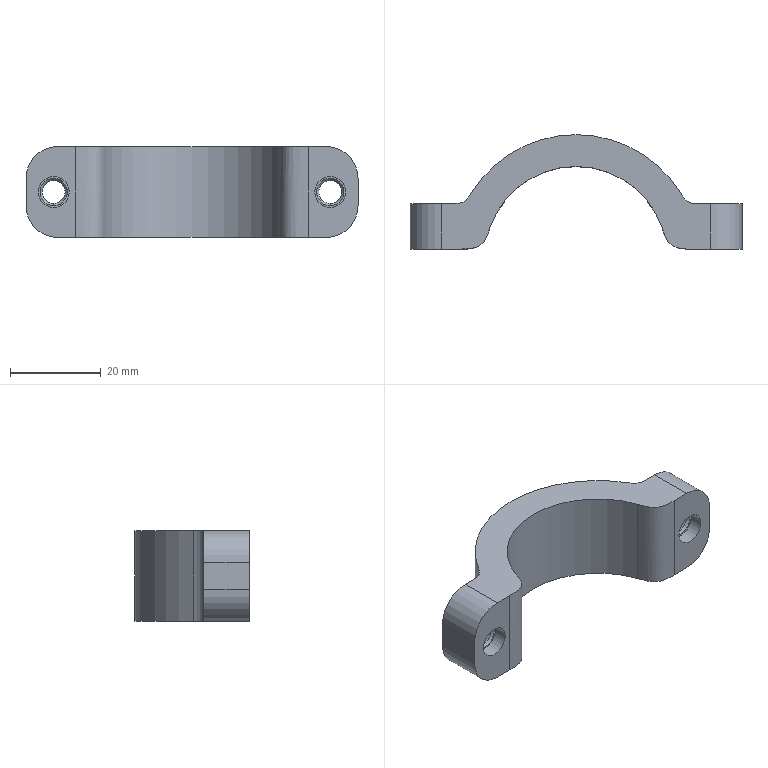Part | 1 solid | 36 faces | box 73 x 25.677 x 20 mm | volume 13024 mm3 | cylinder 14 | plane 10 | cone 8 | other 4 | commonest cylinder face diameters 5 x4 6.8 x4 14 x4 40.1 x1 54.1 x1
STEP:
#1=CARTESIAN_POINT('',(0.,0.,0.));
#2=DIRECTION('',(0.,0.,1.));
#3=DIRECTION('',(1.,0.,0.));
#4=AXIS2_PLACEMENT_3D('',#1,#2,#3);
#5=CARTESIAN_POINT('',(-22.998,-0.2208,0.000000113));
#6=VERTEX_POINT('',#5);
#7=CARTESIAN_POINT('',(-27.249,-2.588,0.000000113));
#8=VERTEX_POINT('',#7);
#9=CARTESIAN_POINT('',(-22.998,-0.2208,0.000000113));
#10=CARTESIAN_POINT('',(-23.584,-1.168,0.000000113));
#11=CARTESIAN_POINT('',(-24.122,-2.145,0.000000113));
#12=CARTESIAN_POINT('',(-25.021,-2.588,0.000000113));
#13=CARTESIAN_POINT('',(-26.135,-2.588,0.000000113));
#14=CARTESIAN_POINT('',(-27.249,-2.588,0.000000113));
#15=B_SPLINE_CURVE_WITH_KNOTS('',5,(#9,#10,#11,#12,#13,#14),.UNSPECIFIED.,.F.,.U.,(6,6),(0.,1.),.UNSPECIFIED.);
#16=EDGE_CURVE('',#6,#8,#15,.T.);
#17=ORIENTED_EDGE('',*,*,#16,.F.);
#18=CARTESIAN_POINT('',(-22.998,-0.2208,-20.));
#19=VERTEX_POINT('',#18);
#20=CARTESIAN_POINT('',(-22.998,-0.2208,-19.5));
#21=DIRECTION('',(0.,0.,1.));
#22=VECTOR('',#21,1.);
#23=LINE('',#20,#22);
#24=EDGE_CURVE('',#19,#6,#23,.T.);
#25=ORIENTED_EDGE('',*,*,#24,.F.);
#26=CARTESIAN_POINT('',(-27.249,-2.588,-20.));
#27=VERTEX_POINT('',#26);
#28=CARTESIAN_POINT('',(-22.998,-0.2208,-20.));
#29=CARTESIAN_POINT('',(-23.584,-1.168,-20.));
#30=CARTESIAN_POINT('',(-24.122,-2.145,-20.));
#31=CARTESIAN_POINT('',(-25.021,-2.588,-20.));
#32=CARTESIAN_POINT('',(-26.135,-2.588,-20.));
#33=CARTESIAN_POINT('',(-27.249,-2.588,-20.));
#34=B_SPLINE_CURVE_WITH_KNOTS('',5,(#28,#29,#30,#31,#32,#33),.UNSPECIFIED.,.F.,.U.,(6,6),(0.,1.),.UNSPECIFIED.);
#35=EDGE_CURVE('',#19,#27,#34,.T.);
#36=ORIENTED_EDGE('',*,*,#35,.T.);
#37=CARTESIAN_POINT('',(-27.249,-2.588,-19.5));
#38=DIRECTION('',(0.,0.,1.));
#39=VECTOR('',#38,1.);
#40=LINE('',#37,#39);
#41=EDGE_CURVE('',#27,#8,#40,.T.);
#42=ORIENTED_EDGE('',*,*,#41,.T.);
#43=EDGE_LOOP('',(#17,#25,#36,#42));
#44=FACE_OUTER_BOUND('',#43,.T.);
#45=CARTESIAN_POINT('',(-22.7,0.2499,-10.));
#46=CARTESIAN_POINT('',(-22.761,0.1563,-10.));
#47=CARTESIAN_POINT('',(-22.821,0.06246,-10.));
#48=CARTESIAN_POINT('',(-22.88,-0.03167,-10.));
#49=CARTESIAN_POINT('',(-23.531,-1.07,-10.));
#50=CARTESIAN_POINT('',(-24.122,-2.145,-10.));
#51=CARTESIAN_POINT('',(-25.021,-2.588,-10.));
#52=CARTESIAN_POINT('',(-26.135,-2.588,-10.));
#53=CARTESIAN_POINT('',(-27.249,-2.588,-10.));
#54=CARTESIAN_POINT('',(-27.36,-2.588,-10.));
#55=CARTESIAN_POINT('',(-27.472,-2.588,-10.));
#56=CARTESIAN_POINT('',(-27.583,-2.588,-10.));
#57=CARTESIAN_POINT('',(-27.694,-2.588,-10.));
#58=CARTESIAN_POINT('',(-27.806,-2.588,-10.));
#59=B_SPLINE_CURVE_WITH_KNOTS('',5,(#45,#46,#47,#48,#49,#50,#51,#52,#53,#54,#55,#56,#57,#58),.UNSPECIFIED.,.F.,.U.,(6,3,5,6),(-0.1,0.,1.,1.1),.UNSPECIFIED.);
#60=DIRECTION('',(0.,0.,1.));
#61=VECTOR('',#60,1.);
#62=SURFACE_OF_LINEAR_EXTRUSION('',#59,#61);
#63=ADVANCED_FACE('',(#44),#62,.T.);
#64=CARTESIAN_POINT('',(22.998,-0.2208,0.000000113));
#65=VERTEX_POINT('',#64);
#66=CARTESIAN_POINT('',(0.000001873,-14.462,0.000000113));
#67=DIRECTION('',(0.,0.,1.));
#68=DIRECTION('',(1.,0.,0.));
#69=AXIS2_PLACEMENT_3D('',#66,#67,#68);
#70=CIRCLE('',#69,27.05);
#71=EDGE_CURVE('',#65,#6,#70,.T.);
#72=ORIENTED_EDGE('',*,*,#71,.F.);
#73=CARTESIAN_POINT('',(22.998,-0.2208,-20.));
#74=VERTEX_POINT('',#73);
#75=CARTESIAN_POINT('',(22.998,-0.2208,-0.5));
#76=DIRECTION('',(0.,0.,-1.));
#77=VECTOR('',#76,1.);
#78=LINE('',#75,#77);
#79=EDGE_CURVE('',#65,#74,#78,.T.);
#80=ORIENTED_EDGE('',*,*,#79,.T.);
#81=CARTESIAN_POINT('',(0.000001873,-14.462,-20.));
#82=DIRECTION('',(0.,0.,1.));
#83=DIRECTION('',(-1.,0.,0.));
#84=AXIS2_PLACEMENT_3D('',#81,#82,#83);
#85=CIRCLE('',#84,27.05);
#86=EDGE_CURVE('',#74,#19,#85,.T.);
#87=ORIENTED_EDGE('',*,*,#86,.T.);
#88=ORIENTED_EDGE('',*,*,#24,.T.);
#89=EDGE_LOOP('',(#72,#80,#87,#88));
#90=FACE_OUTER_BOUND('',#89,.T.);
#91=CARTESIAN_POINT('',(0.000001873,-14.462,0.45));
#92=DIRECTION('',(0.,0.,-1.));
#93=DIRECTION('',(0.,-1.,0.));
#94=AXIS2_PLACEMENT_3D('',#91,#92,#93);
#95=CYLINDRICAL_SURFACE('',#94,27.05);
#96=ADVANCED_FACE('',(#90),#95,.T.);
#97=CARTESIAN_POINT('',(27.249,-2.588,0.000000113));
#98=VERTEX_POINT('',#97);
#99=CARTESIAN_POINT('',(27.249,-2.588,0.000000113));
#100=CARTESIAN_POINT('',(26.135,-2.588,0.000000113));
#101=CARTESIAN_POINT('',(25.021,-2.588,0.000000113));
#102=CARTESIAN_POINT('',(24.122,-2.145,0.000000113));
#103=CARTESIAN_POINT('',(23.584,-1.168,0.000000113));
#104=CARTESIAN_POINT('',(22.998,-0.2208,0.000000113));
#105=B_SPLINE_CURVE_WITH_KNOTS('',5,(#99,#100,#101,#102,#103,#104),.UNSPECIFIED.,.F.,.U.,(6,6),(0.,1.),.UNSPECIFIED.);
#106=EDGE_CURVE('',#98,#65,#105,.T.);
#107=ORIENTED_EDGE('',*,*,#106,.F.);
#108=CARTESIAN_POINT('',(27.249,-2.588,-20.));
#109=VERTEX_POINT('',#108);
#110=CARTESIAN_POINT('',(27.249,-2.588,-0.5));
#111=DIRECTION('',(0.,0.,-1.));
#112=VECTOR('',#111,1.);
#113=LINE('',#110,#112);
#114=EDGE_CURVE('',#98,#109,#113,.T.);
#115=ORIENTED_EDGE('',*,*,#114,.T.);
#116=CARTESIAN_POINT('',(27.249,-2.588,-20.));
#117=CARTESIAN_POINT('',(26.135,-2.588,-20.));
#118=CARTESIAN_POINT('',(25.021,-2.588,-20.));
#119=CARTESIAN_POINT('',(24.122,-2.145,-20.));
#120=CARTESIAN_POINT('',(23.584,-1.168,-20.));
#121=CARTESIAN_POINT('',(22.998,-0.2208,-20.));
#122=B_SPLINE_CURVE_WITH_KNOTS('',5,(#116,#117,#118,#119,#120,#121),.UNSPECIFIED.,.F.,.U.,(6,6),(0.,1.),.UNSPECIFIED.);
#123=EDGE_CURVE('',#109,#74,#122,.T.);
#124=ORIENTED_EDGE('',*,*,#123,.T.);
#125=ORIENTED_EDGE('',*,*,#79,.F.);
#126=EDGE_LOOP('',(#107,#115,#124,#125));
#127=FACE_OUTER_BOUND('',#126,.T.);
#128=CARTESIAN_POINT('',(27.806,-2.588,-10.));
#129=CARTESIAN_POINT('',(27.694,-2.588,-10.));
#130=CARTESIAN_POINT('',(27.583,-2.588,-10.));
#131=CARTESIAN_POINT('',(27.472,-2.588,-10.));
#132=CARTESIAN_POINT('',(27.36,-2.588,-10.));
#133=CARTESIAN_POINT('',(27.249,-2.588,-10.));
#134=CARTESIAN_POINT('',(26.135,-2.588,-10.));
#135=CARTESIAN_POINT('',(25.021,-2.588,-10.));
#136=CARTESIAN_POINT('',(24.122,-2.145,-10.));
#137=CARTESIAN_POINT('',(23.531,-1.07,-10.));
#138=CARTESIAN_POINT('',(22.88,-0.03167,-10.));
#139=CARTESIAN_POINT('',(22.821,0.06246,-10.));
#140=CARTESIAN_POINT('',(22.761,0.1563,-10.));
#141=CARTESIAN_POINT('',(22.7,0.2499,-10.));
#142=B_SPLINE_CURVE_WITH_KNOTS('',5,(#128,#129,#130,#131,#132,#133,#134,#135,#136,#137,#138,#139,#140,#141),.UNSPECIFIED.,.F.,.U.,(6,5,3,6),(-0.1,0.,1.,1.1),.UNSPECIFIED.);
#143=DIRECTION('',(0.,0.,1.));
#144=VECTOR('',#143,1.);
#145=SURFACE_OF_LINEAR_EXTRUSION('',#142,#144);
#146=ADVANCED_FACE('',(#127),#145,.T.);
#147=CARTESIAN_POINT('',(-36.5,-2.588,-7.));
#148=VERTEX_POINT('',#147);
#149=CARTESIAN_POINT('',(-29.5,-2.588,0.000000113));
#150=VERTEX_POINT('',#149);
#151=CARTESIAN_POINT('',(-29.5,-2.588,-7.));
#152=DIRECTION('',(0.,1.,0.));
#153=DIRECTION('',(-1.,0.,0.));
#154=AXIS2_PLACEMENT_3D('',#151,#152,#153);
#155=CIRCLE('',#154,7.);
#156=EDGE_CURVE('',#148,#150,#155,.T.);
#157=ORIENTED_EDGE('',*,*,#156,.F.);
#158=CARTESIAN_POINT('',(-36.5,-12.588,-7.));
#159=VERTEX_POINT('',#158);
#160=CARTESIAN_POINT('',(-36.5,-3.088,-7.));
#161=DIRECTION('',(0.,-1.,0.));
#162=VECTOR('',#161,1.);
#163=LINE('',#160,#162);
#164=EDGE_CURVE('',#148,#159,#163,.T.);
#165=ORIENTED_EDGE('',*,*,#164,.T.);
#166=CARTESIAN_POINT('',(-29.5,-12.588,0.000000113));
#167=VERTEX_POINT('',#166);
#168=CARTESIAN_POINT('',(-29.5,-12.588,-7.));
#169=DIRECTION('',(0.,1.,0.));
#170=DIRECTION('',(1.,0.,0.));
#171=AXIS2_PLACEMENT_3D('',#168,#169,#170);
#172=CIRCLE('',#171,7.);
#173=EDGE_CURVE('',#159,#167,#172,.T.);
#174=ORIENTED_EDGE('',*,*,#173,.T.);
#175=CARTESIAN_POINT('',(-29.5,-3.088,0.000000113));
#176=DIRECTION('',(0.,-1.,0.));
#177=VECTOR('',#176,1.);
#178=LINE('',#175,#177);
#179=EDGE_CURVE('',#150,#167,#178,.T.);
#180=ORIENTED_EDGE('',*,*,#179,.F.);
#181=EDGE_LOOP('',(#157,#165,#174,#180));
#182=FACE_OUTER_BOUND('',#181,.T.);
#183=CARTESIAN_POINT('',(-29.5,-12.538,-7.));
#184=DIRECTION('',(0.,1.,0.));
#185=DIRECTION('',(0.7071,0.,-0.7071));
#186=AXIS2_PLACEMENT_3D('',#183,#184,#185);
#187=CYLINDRICAL_SURFACE('',#186,7.);
#188=ADVANCED_FACE('',(#182),#187,.T.);
#189=CARTESIAN_POINT('',(-36.5,-2.588,-13.));
#190=VERTEX_POINT('',#189);
#191=CARTESIAN_POINT('',(-36.5,-2.588,0.45));
#192=DIRECTION('',(0.,0.,1.));
#193=VECTOR('',#192,1.);
#194=LINE('',#191,#193);
#195=EDGE_CURVE('',#190,#148,#194,.T.);
#196=ORIENTED_EDGE('',*,*,#195,.F.);
#197=CARTESIAN_POINT('',(-36.5,-12.588,-13.));
#198=VERTEX_POINT('',#197);
#199=CARTESIAN_POINT('',(-36.5,-12.088,-13.));
#200=DIRECTION('',(0.,1.,0.));
#201=VECTOR('',#200,1.);
#202=LINE('',#199,#201);
#203=EDGE_CURVE('',#198,#190,#202,.T.);
#204=ORIENTED_EDGE('',*,*,#203,.F.);
#205=CARTESIAN_POINT('',(-36.5,-12.588,-13.3));
#206=DIRECTION('',(0.,0.,1.));
#207=VECTOR('',#206,1.);
#208=LINE('',#205,#207);
#209=EDGE_CURVE('',#198,#159,#208,.T.);
#210=ORIENTED_EDGE('',*,*,#209,.T.);
#211=ORIENTED_EDGE('',*,*,#164,.F.);
#212=EDGE_LOOP('',(#196,#204,#210,#211));
#213=FACE_OUTER_BOUND('',#212,.T.);
#214=CARTESIAN_POINT('',(-36.5,-12.538,-13.3));
#215=DIRECTION('',(-1.,0.,0.));
#216=DIRECTION('',(0.,0.,1.));
#217=AXIS2_PLACEMENT_3D('',#214,#215,#216);
#218=PLANE('',#217);
#219=ADVANCED_FACE('',(#213),#218,.T.);
#220=CARTESIAN_POINT('',(-29.5,-2.588,-20.));
#221=VERTEX_POINT('',#220);
#222=CARTESIAN_POINT('',(-29.5,-2.588,-13.));
#223=DIRECTION('',(0.,1.,0.));
#224=DIRECTION('',(-1.,0.,0.));
#225=AXIS2_PLACEMENT_3D('',#222,#223,#224);
#226=CIRCLE('',#225,7.);
#227=EDGE_CURVE('',#221,#190,#226,.T.);
#228=ORIENTED_EDGE('',*,*,#227,.F.);
#229=CARTESIAN_POINT('',(-29.5,-12.588,-20.));
#230=VERTEX_POINT('',#229);
#231=CARTESIAN_POINT('',(-29.5,-12.088,-20.));
#232=DIRECTION('',(0.,1.,0.));
#233=VECTOR('',#232,1.);
#234=LINE('',#231,#233);
#235=EDGE_CURVE('',#230,#221,#234,.T.);
#236=ORIENTED_EDGE('',*,*,#235,.F.);
#237=CARTESIAN_POINT('',(-29.5,-12.588,-13.));
#238=DIRECTION('',(0.,1.,0.));
#239=DIRECTION('',(1.,0.,0.));
#240=AXIS2_PLACEMENT_3D('',#237,#238,#239);
#241=CIRCLE('',#240,7.);
#242=EDGE_CURVE('',#230,#198,#241,.T.);
#243=ORIENTED_EDGE('',*,*,#242,.T.);
#244=ORIENTED_EDGE('',*,*,#203,.T.);
#245=EDGE_LOOP('',(#228,#236,#243,#244));
#246=FACE_OUTER_BOUND('',#245,.T.);
#247=CARTESIAN_POINT('',(-29.5,-2.638,-13.));
#248=DIRECTION('',(0.,-1.,0.));
#249=DIRECTION('',(0.7071,0.,0.7071));
#250=AXIS2_PLACEMENT_3D('',#247,#248,#249);
#251=CYLINDRICAL_SURFACE('',#250,7.);
#252=ADVANCED_FACE('',(#246),#251,.T.);
#253=CARTESIAN_POINT('',(-26.811,-2.588,-20.));
#254=DIRECTION('',(-1.,0.,0.));
#255=VECTOR('',#254,1.);
#256=LINE('',#253,#255);
#257=EDGE_CURVE('',#27,#221,#256,.T.);
#258=ORIENTED_EDGE('',*,*,#257,.F.);
#259=ORIENTED_EDGE('',*,*,#35,.F.);
#260=ORIENTED_EDGE('',*,*,#86,.F.);
#261=ORIENTED_EDGE('',*,*,#123,.F.);
#262=CARTESIAN_POINT('',(29.5,-2.588,-20.));
#263=VERTEX_POINT('',#262);
#264=CARTESIAN_POINT('',(36.438,-2.588,-20.));
#265=DIRECTION('',(-1.,0.,0.));
#266=VECTOR('',#265,1.);
#267=LINE('',#264,#266);
#268=EDGE_CURVE('',#263,#109,#267,.T.);
#269=ORIENTED_EDGE('',*,*,#268,.F.);
#270=CARTESIAN_POINT('',(29.5,-12.588,-20.));
#271=VERTEX_POINT('',#270);
#272=CARTESIAN_POINT('',(29.5,-3.088,-20.));
#273=DIRECTION('',(0.,-1.,0.));
#274=VECTOR('',#273,1.);
#275=LINE('',#272,#274);
#276=EDGE_CURVE('',#263,#271,#275,.T.);
#277=ORIENTED_EDGE('',*,*,#276,.T.);
#278=CARTESIAN_POINT('',(25.553,-12.588,-20.));
#279=VERTEX_POINT('',#278);
#280=CARTESIAN_POINT('',(45.625,-12.588,-20.));
#281=DIRECTION('',(-1.,0.,0.));
#282=VECTOR('',#281,1.);
#283=LINE('',#280,#282);
#284=EDGE_CURVE('',#271,#279,#283,.T.);
#285=ORIENTED_EDGE('',*,*,#284,.T.);
#286=CARTESIAN_POINT('',(18.941,-7.885,-20.));
#287=VERTEX_POINT('',#286);
#288=CARTESIAN_POINT('',(25.553,-12.588,-20.));
#289=CARTESIAN_POINT('',(23.562,-12.588,-20.));
#290=CARTESIAN_POINT('',(21.57,-12.588,-20.));
#291=CARTESIAN_POINT('',(20.014,-11.729,-20.));
#292=CARTESIAN_POINT('',(19.594,-9.766,-20.));
#293=CARTESIAN_POINT('',(18.941,-7.885,-20.));
#294=B_SPLINE_CURVE_WITH_KNOTS('',5,(#288,#289,#290,#291,#292,#293),.UNSPECIFIED.,.F.,.U.,(6,6),(0.,1.),.UNSPECIFIED.);
#295=EDGE_CURVE('',#279,#287,#294,.T.);
#296=ORIENTED_EDGE('',*,*,#295,.T.);
#297=CARTESIAN_POINT('',(-18.941,-7.885,-20.));
#298=VERTEX_POINT('',#297);
#299=CARTESIAN_POINT('',(0.000001873,-14.462,-20.));
#300=DIRECTION('',(0.,0.,-1.));
#301=DIRECTION('',(-1.,0.,0.));
#302=AXIS2_PLACEMENT_3D('',#299,#300,#301);
#303=CIRCLE('',#302,20.05);
#304=EDGE_CURVE('',#298,#287,#303,.T.);
#305=ORIENTED_EDGE('',*,*,#304,.F.);
#306=CARTESIAN_POINT('',(-25.553,-12.588,-20.));
#307=VERTEX_POINT('',#306);
#308=CARTESIAN_POINT('',(-18.941,-7.885,-20.));
#309=CARTESIAN_POINT('',(-19.594,-9.766,-20.));
#310=CARTESIAN_POINT('',(-20.014,-11.729,-20.));
#311=CARTESIAN_POINT('',(-21.57,-12.588,-20.));
#312=CARTESIAN_POINT('',(-23.562,-12.588,-20.));
#313=CARTESIAN_POINT('',(-25.553,-12.588,-20.));
#314=B_SPLINE_CURVE_WITH_KNOTS('',5,(#308,#309,#310,#311,#312,#313),.UNSPECIFIED.,.F.,.U.,(6,6),(0.,1.),.UNSPECIFIED.);
#315=EDGE_CURVE('',#298,#307,#314,.T.);
#316=ORIENTED_EDGE('',*,*,#315,.T.);
#317=CARTESIAN_POINT('',(45.625,-12.588,-20.));
#318=DIRECTION('',(-1.,0.,0.));
#319=VECTOR('',#318,1.);
#320=LINE('',#317,#319);
#321=EDGE_CURVE('',#307,#230,#320,.T.);
#322=ORIENTED_EDGE('',*,*,#321,.T.);
#323=ORIENTED_EDGE('',*,*,#235,.T.);
#324=EDGE_LOOP('',(#258,#259,#260,#261,#269,#277,#285,#296,#305,#316,#322,#323));
#325=FACE_OUTER_BOUND('',#324,.T.);
#326=CARTESIAN_POINT('',(45.625,15.736,-20.));
#327=DIRECTION('',(0.,0.,-1.));
#328=DIRECTION('',(0.,-1.,0.));
#329=AXIS2_PLACEMENT_3D('',#326,#327,#328);
#330=PLANE('',#329);
#331=ADVANCED_FACE('',(#325),#330,.T.);
#332=CARTESIAN_POINT('',(30.4,-2.588,-13.));
#333=VERTEX_POINT('',#332);
#334=CARTESIAN_POINT('',(30.4,-2.588,-7.));
#335=VERTEX_POINT('',#334);
#336=CARTESIAN_POINT('',(30.4,-2.588,-10.));
#337=DIRECTION('',(0.,-1.,0.));
#338=DIRECTION('',(0.,0.,-1.));
#339=AXIS2_PLACEMENT_3D('',#336,#337,#338);
#340=CIRCLE('',#339,3.);
#341=EDGE_CURVE('',#333,#335,#340,.T.);
#342=ORIENTED_EDGE('',*,*,#341,.T.);
#343=CARTESIAN_POINT('',(30.4,-2.588,-10.));
#344=DIRECTION('',(0.,-1.,0.));
#345=DIRECTION('',(0.,0.,-1.));
#346=AXIS2_PLACEMENT_3D('',#343,#344,#345);
#347=CIRCLE('',#346,3.);
#348=EDGE_CURVE('',#335,#333,#347,.T.);
#349=ORIENTED_EDGE('',*,*,#348,.T.);
#350=EDGE_LOOP('',(#342,#349));
#351=FACE_BOUND('',#350,.T.);
#352=ORIENTED_EDGE('',*,*,#114,.F.);
#353=CARTESIAN_POINT('',(29.5,-2.588,0.000000113));
#354=VERTEX_POINT('',#353);
#355=CARTESIAN_POINT('',(36.438,-2.588,0.000000113));
#356=DIRECTION('',(1.,0.,0.));
#357=VECTOR('',#356,1.);
#358=LINE('',#355,#357);
#359=EDGE_CURVE('',#98,#354,#358,.T.);
#360=ORIENTED_EDGE('',*,*,#359,.T.);
#361=CARTESIAN_POINT('',(36.5,-2.588,-7.));
#362=VERTEX_POINT('',#361);
#363=CARTESIAN_POINT('',(29.5,-2.588,-7.));
#364=DIRECTION('',(0.,1.,0.));
#365=DIRECTION('',(-1.,0.,0.));
#366=AXIS2_PLACEMENT_3D('',#363,#364,#365);
#367=CIRCLE('',#366,7.);
#368=EDGE_CURVE('',#354,#362,#367,.T.);
#369=ORIENTED_EDGE('',*,*,#368,.T.);
#370=CARTESIAN_POINT('',(36.5,-2.588,-13.));
#371=VERTEX_POINT('',#370);
#372=CARTESIAN_POINT('',(36.5,-2.588,0.45));
#373=DIRECTION('',(0.,0.,-1.));
#374=VECTOR('',#373,1.);
#375=LINE('',#372,#374);
#376=EDGE_CURVE('',#362,#371,#375,.T.);
#377=ORIENTED_EDGE('',*,*,#376,.T.);
#378=CARTESIAN_POINT('',(29.5,-2.588,-13.));
#379=DIRECTION('',(0.,1.,0.));
#380=DIRECTION('',(-1.,0.,0.));
#381=AXIS2_PLACEMENT_3D('',#378,#379,#380);
#382=CIRCLE('',#381,7.);
#383=EDGE_CURVE('',#371,#263,#382,.T.);
#384=ORIENTED_EDGE('',*,*,#383,.T.);
#385=ORIENTED_EDGE('',*,*,#268,.T.);
#386=EDGE_LOOP('',(#352,#360,#369,#377,#384,#385));
#387=FACE_OUTER_BOUND('',#386,.T.);
#388=CARTESIAN_POINT('',(36.438,-2.588,0.45));
#389=DIRECTION('',(0.,1.,0.));
#390=DIRECTION('',(0.,0.,-1.));
#391=AXIS2_PLACEMENT_3D('',#388,#389,#390);
#392=PLANE('',#391);
#393=ADVANCED_FACE('',(#351,#387),#392,.T.);
#394=ORIENTED_EDGE('',*,*,#383,.F.);
#395=CARTESIAN_POINT('',(36.5,-12.588,-13.));
#396=VERTEX_POINT('',#395);
#397=CARTESIAN_POINT('',(36.5,-3.088,-13.));
#398=DIRECTION('',(0.,-1.,0.));
#399=VECTOR('',#398,1.);
#400=LINE('',#397,#399);
#401=EDGE_CURVE('',#371,#396,#400,.T.);
#402=ORIENTED_EDGE('',*,*,#401,.T.);
#403=CARTESIAN_POINT('',(29.5,-12.588,-13.));
#404=DIRECTION('',(0.,1.,0.));
#405=DIRECTION('',(1.,0.,0.));
#406=AXIS2_PLACEMENT_3D('',#403,#404,#405);
#407=CIRCLE('',#406,7.);
#408=EDGE_CURVE('',#396,#271,#407,.T.);
#409=ORIENTED_EDGE('',*,*,#408,.T.);
#410=ORIENTED_EDGE('',*,*,#276,.F.);
#411=EDGE_LOOP('',(#394,#402,#409,#410));
#412=FACE_OUTER_BOUND('',#411,.T.);
#413=CARTESIAN_POINT('',(29.5,-12.538,-13.));
#414=DIRECTION('',(0.,1.,0.));
#415=DIRECTION('',(-0.7071,0.,0.7071));
#416=AXIS2_PLACEMENT_3D('',#413,#414,#415);
#417=CYLINDRICAL_SURFACE('',#416,7.);
#418=ADVANCED_FACE('',(#412),#417,.T.);
#419=ORIENTED_EDGE('',*,*,#376,.F.);
#420=CARTESIAN_POINT('',(36.5,-12.588,-7.));
#421=VERTEX_POINT('',#420);
#422=CARTESIAN_POINT('',(36.5,-12.088,-7.));
#423=DIRECTION('',(0.,1.,0.));
#424=VECTOR('',#423,1.);
#425=LINE('',#422,#424);
#426=EDGE_CURVE('',#421,#362,#425,.T.);
#427=ORIENTED_EDGE('',*,*,#426,.F.);
#428=CARTESIAN_POINT('',(36.5,-12.588,-6.7));
#429=DIRECTION('',(0.,0.,-1.));
#430=VECTOR('',#429,1.);
#431=LINE('',#428,#430);
#432=EDGE_CURVE('',#421,#396,#431,.T.);
#433=ORIENTED_EDGE('',*,*,#432,.T.);
#434=ORIENTED_EDGE('',*,*,#401,.F.);
#435=EDGE_LOOP('',(#419,#427,#433,#434));
#436=FACE_OUTER_BOUND('',#435,.T.);
#437=CARTESIAN_POINT('',(36.5,-12.538,-6.7));
#438=DIRECTION('',(1.,0.,0.));
#439=DIRECTION('',(0.,0.,-1.));
#440=AXIS2_PLACEMENT_3D('',#437,#438,#439);
#441=PLANE('',#440);
#442=ADVANCED_FACE('',(#436),#441,.T.);
#443=ORIENTED_EDGE('',*,*,#368,.F.);
#444=CARTESIAN_POINT('',(29.5,-12.588,0.000000113));
#445=VERTEX_POINT('',#444);
#446=CARTESIAN_POINT('',(29.5,-12.088,0.000000113));
#447=DIRECTION('',(0.,1.,0.));
#448=VECTOR('',#447,1.);
#449=LINE('',#446,#448);
#450=EDGE_CURVE('',#445,#354,#449,.T.);
#451=ORIENTED_EDGE('',*,*,#450,.F.);
#452=CARTESIAN_POINT('',(29.5,-12.588,-7.));
#453=DIRECTION('',(0.,1.,0.));
#454=DIRECTION('',(1.,0.,0.));
#455=AXIS2_PLACEMENT_3D('',#452,#453,#454);
#456=CIRCLE('',#455,7.);
#457=EDGE_CURVE('',#445,#421,#456,.T.);
#458=ORIENTED_EDGE('',*,*,#457,.T.);
#459=ORIENTED_EDGE('',*,*,#426,.T.);
#460=EDGE_LOOP('',(#443,#451,#458,#459));
#461=FACE_OUTER_BOUND('',#460,.T.);
#462=CARTESIAN_POINT('',(29.5,-2.638,-7.));
#463=DIRECTION('',(0.,-1.,0.));
#464=DIRECTION('',(-0.7071,0.,-0.7071));
#465=AXIS2_PLACEMENT_3D('',#462,#463,#464);
#466=CYLINDRICAL_SURFACE('',#465,7.);
#467=ADVANCED_FACE('',(#461),#466,.T.);
#468=ORIENTED_EDGE('',*,*,#71,.T.);
#469=ORIENTED_EDGE('',*,*,#16,.T.);
#470=CARTESIAN_POINT('',(-26.811,-2.588,0.000000113));
#471=DIRECTION('',(1.,0.,0.));
#472=VECTOR('',#471,1.);
#473=LINE('',#470,#472);
#474=EDGE_CURVE('',#150,#8,#473,.T.);
#475=ORIENTED_EDGE('',*,*,#474,.F.);
#476=ORIENTED_EDGE('',*,*,#179,.T.);
#477=CARTESIAN_POINT('',(-25.553,-12.588,0.000000113));
#478=VERTEX_POINT('',#477);
#479=CARTESIAN_POINT('',(32.45,-12.588,0.000000113));
#480=DIRECTION('',(1.,0.,0.));
#481=VECTOR('',#480,1.);
#482=LINE('',#479,#481);
#483=EDGE_CURVE('',#167,#478,#482,.T.);
#484=ORIENTED_EDGE('',*,*,#483,.T.);
#485=CARTESIAN_POINT('',(-18.941,-7.885,0.000000113));
#486=VERTEX_POINT('',#485);
#487=CARTESIAN_POINT('',(-25.553,-12.588,0.000000113));
#488=CARTESIAN_POINT('',(-23.562,-12.588,0.000000113));
#489=CARTESIAN_POINT('',(-21.57,-12.588,0.000000113));
#490=CARTESIAN_POINT('',(-20.014,-11.729,0.000000113));
#491=CARTESIAN_POINT('',(-19.594,-9.766,0.000000113));
#492=CARTESIAN_POINT('',(-18.941,-7.885,0.000000113));
#493=B_SPLINE_CURVE_WITH_KNOTS('',5,(#487,#488,#489,#490,#491,#492),.UNSPECIFIED.,.F.,.U.,(6,6),(0.,1.),.UNSPECIFIED.);
#494=EDGE_CURVE('',#478,#486,#493,.T.);
#495=ORIENTED_EDGE('',*,*,#494,.T.);
#496=CARTESIAN_POINT('',(18.941,-7.885,0.000000113));
#497=VERTEX_POINT('',#496);
#498=CARTESIAN_POINT('',(0.000001873,-14.462,0.000000113));
#499=DIRECTION('',(0.,0.,1.));
#500=DIRECTION('',(1.,0.,0.));
#501=AXIS2_PLACEMENT_3D('',#498,#499,#500);
#502=CIRCLE('',#501,20.05);
#503=EDGE_CURVE('',#497,#486,#502,.T.);
#504=ORIENTED_EDGE('',*,*,#503,.F.);
#505=CARTESIAN_POINT('',(25.553,-12.588,0.000000113));
#506=VERTEX_POINT('',#505);
#507=CARTESIAN_POINT('',(18.941,-7.885,0.000000113));
#508=CARTESIAN_POINT('',(19.594,-9.766,0.000000113));
#509=CARTESIAN_POINT('',(20.014,-11.729,0.000000113));
#510=CARTESIAN_POINT('',(21.57,-12.588,0.000000113));
#511=CARTESIAN_POINT('',(23.562,-12.588,0.000000113));
#512=CARTESIAN_POINT('',(25.553,-12.588,0.000000113));
#513=B_SPLINE_CURVE_WITH_KNOTS('',5,(#507,#508,#509,#510,#511,#512),.UNSPECIFIED.,.F.,.U.,(6,6),(0.,1.),.UNSPECIFIED.);
#514=EDGE_CURVE('',#497,#506,#513,.T.);
#515=ORIENTED_EDGE('',*,*,#514,.T.);
#516=CARTESIAN_POINT('',(32.45,-12.588,0.000000113));
#517=DIRECTION('',(1.,0.,0.));
#518=VECTOR('',#517,1.);
#519=LINE('',#516,#518);
#520=EDGE_CURVE('',#506,#445,#519,.T.);
#521=ORIENTED_EDGE('',*,*,#520,.T.);
#522=ORIENTED_EDGE('',*,*,#450,.T.);
#523=ORIENTED_EDGE('',*,*,#359,.F.);
#524=ORIENTED_EDGE('',*,*,#106,.T.);
#525=EDGE_LOOP('',(#468,#469,#475,#476,#484,#495,#504,#515,#521,#522,#523,#524));
#526=FACE_OUTER_BOUND('',#525,.T.);
#527=CARTESIAN_POINT('',(32.45,-13.297,0.000000113));
#528=DIRECTION('',(0.,0.,1.));
#529=DIRECTION('',(0.,1.,0.));
#530=AXIS2_PLACEMENT_3D('',#527,#528,#529);
#531=PLANE('',#530);
#532=ADVANCED_FACE('',(#526),#531,.T.);
#533=CARTESIAN_POINT('',(30.4,-3.088,-7.5));
#534=VERTEX_POINT('',#533);
#535=CARTESIAN_POINT('',(30.4,-3.088,-7.5));
#536=DIRECTION('',(0.,0.7071,0.7071));
#537=VECTOR('',#536,1.);
#538=LINE('',#535,#537);
#539=EDGE_CURVE('',#534,#335,#538,.T.);
#540=ORIENTED_EDGE('',*,*,#539,.T.);
#541=ORIENTED_EDGE('',*,*,#341,.F.);
#542=CARTESIAN_POINT('',(30.4,-3.088,-12.5));
#543=VERTEX_POINT('',#542);
#544=CARTESIAN_POINT('',(30.4,-3.088,-12.5));
#545=DIRECTION('',(0.,0.7071,-0.7071));
#546=VECTOR('',#545,1.);
#547=LINE('',#544,#546);
#548=EDGE_CURVE('',#543,#333,#547,.T.);
#549=ORIENTED_EDGE('',*,*,#548,.F.);
#550=CARTESIAN_POINT('',(31.247,-3.088,-12.352));
#551=VERTEX_POINT('',#550);
#552=CARTESIAN_POINT('',(30.4,-3.088,-10.));
#553=DIRECTION('',(0.,1.,0.));
#554=DIRECTION('',(0.,0.,1.));
#555=AXIS2_PLACEMENT_3D('',#552,#553,#554);
#556=CIRCLE('',#555,2.5);
#557=EDGE_CURVE('',#551,#543,#556,.T.);
#558=ORIENTED_EDGE('',*,*,#557,.F.);
#559=CARTESIAN_POINT('',(30.4,-3.088,-10.));
#560=DIRECTION('',(0.,1.,0.));
#561=DIRECTION('',(0.,0.,1.));
#562=AXIS2_PLACEMENT_3D('',#559,#560,#561);
#563=CIRCLE('',#562,2.5);
#564=EDGE_CURVE('',#534,#551,#563,.T.);
#565=ORIENTED_EDGE('',*,*,#564,.F.);
#566=EDGE_LOOP('',(#540,#541,#549,#558,#565));
#567=FACE_OUTER_BOUND('',#566,.T.);
#568=CARTESIAN_POINT('',(30.4,-3.113,-10.));
#569=DIRECTION('',(0.,1.,0.));
#570=DIRECTION('',(-1.,0.,0.));
#571=AXIS2_PLACEMENT_3D('',#568,#569,#570);
#572=CONICAL_SURFACE('',#571,2.475,0.7854);
#573=ADVANCED_FACE('',(#567),#572,.F.);
#574=CARTESIAN_POINT('',(-30.4,-3.088,-7.5));
#575=VERTEX_POINT('',#574);
#576=CARTESIAN_POINT('',(-30.4,-2.588,-7.));
#577=VERTEX_POINT('',#576);
#578=CARTESIAN_POINT('',(-30.4,-3.088,-7.5));
#579=DIRECTION('',(0.,0.7071,0.7071));
#580=VECTOR('',#579,1.);
#581=LINE('',#578,#580);
#582=EDGE_CURVE('',#575,#577,#581,.T.);
#583=ORIENTED_EDGE('',*,*,#582,.T.);
#584=CARTESIAN_POINT('',(-30.4,-2.588,-13.));
#585=VERTEX_POINT('',#584);
#586=CARTESIAN_POINT('',(-30.4,-2.588,-10.));
#587=DIRECTION('',(0.,-1.,0.));
#588=DIRECTION('',(0.,0.,-1.));
#589=AXIS2_PLACEMENT_3D('',#586,#587,#588);
#590=CIRCLE('',#589,3.);
#591=EDGE_CURVE('',#585,#577,#590,.T.);
#592=ORIENTED_EDGE('',*,*,#591,.F.);
#593=CARTESIAN_POINT('',(-30.4,-3.088,-12.5));
#594=VERTEX_POINT('',#593);
#595=CARTESIAN_POINT('',(-30.4,-3.088,-12.5));
#596=DIRECTION('',(0.,0.7071,-0.7071));
#597=VECTOR('',#596,1.);
#598=LINE('',#595,#597);
#599=EDGE_CURVE('',#594,#585,#598,.T.);
#600=ORIENTED_EDGE('',*,*,#599,.F.);
#601=CARTESIAN_POINT('',(-29.553,-3.088,-12.352));
#602=VERTEX_POINT('',#601);
#603=CARTESIAN_POINT('',(-30.4,-3.088,-10.));
#604=DIRECTION('',(0.,1.,0.));
#605=DIRECTION('',(0.,0.,1.));
#606=AXIS2_PLACEMENT_3D('',#603,#604,#605);
#607=CIRCLE('',#606,2.5);
#608=EDGE_CURVE('',#602,#594,#607,.T.);
#609=ORIENTED_EDGE('',*,*,#608,.F.);
#610=CARTESIAN_POINT('',(-30.4,-3.088,-10.));
#611=DIRECTION('',(0.,1.,0.));
#612=DIRECTION('',(0.,0.,1.));
#613=AXIS2_PLACEMENT_3D('',#610,#611,#612);
#614=CIRCLE('',#613,2.5);
#615=EDGE_CURVE('',#575,#602,#614,.T.);
#616=ORIENTED_EDGE('',*,*,#615,.F.);
#617=EDGE_LOOP('',(#583,#592,#600,#609,#616));
#618=FACE_OUTER_BOUND('',#617,.T.);
#619=CARTESIAN_POINT('',(-30.4,-3.113,-10.));
#620=DIRECTION('',(0.,1.,0.));
#621=DIRECTION('',(-1.,0.,0.));
#622=AXIS2_PLACEMENT_3D('',#619,#620,#621);
#623=CONICAL_SURFACE('',#622,2.475,0.7854);
#624=ADVANCED_FACE('',(#618),#623,.F.);
#625=CARTESIAN_POINT('',(18.941,-7.885,-0.5));
#626=DIRECTION('',(0.,0.,-1.));
#627=VECTOR('',#626,1.);
#628=LINE('',#625,#627);
#629=EDGE_CURVE('',#497,#287,#628,.T.);
#630=ORIENTED_EDGE('',*,*,#629,.F.);
#631=ORIENTED_EDGE('',*,*,#503,.T.);
#632=CARTESIAN_POINT('',(-18.941,-7.885,-19.5));
#633=DIRECTION('',(0.,0.,1.));
#634=VECTOR('',#633,1.);
#635=LINE('',#632,#634);
#636=EDGE_CURVE('',#298,#486,#635,.T.);
#637=ORIENTED_EDGE('',*,*,#636,.F.);
#638=ORIENTED_EDGE('',*,*,#304,.T.);
#639=EDGE_LOOP('',(#630,#631,#637,#638));
#640=FACE_OUTER_BOUND('',#639,.T.);
#641=CARTESIAN_POINT('',(0.000001873,-14.462,-20.45));
#642=DIRECTION('',(0.,0.,1.));
#643=DIRECTION('',(0.,-1.,0.));
#644=AXIS2_PLACEMENT_3D('',#641,#642,#643);
#645=CYLINDRICAL_SURFACE('',#644,20.05);
#646=ADVANCED_FACE('',(#640),#645,.F.);
#647=CARTESIAN_POINT('',(31.247,-9.088,-12.352));
#648=VERTEX_POINT('',#647);
#649=CARTESIAN_POINT('',(31.247,-3.088,-12.352));
#650=DIRECTION('',(0.,-1.,0.));
#651=VECTOR('',#650,1.);
#652=LINE('',#649,#651);
#653=EDGE_CURVE('',#551,#648,#652,.T.);
#654=ORIENTED_EDGE('',*,*,#653,.T.);
#655=CARTESIAN_POINT('',(30.4,-9.088,-7.5));
#656=VERTEX_POINT('',#655);
#657=CARTESIAN_POINT('',(30.4,-9.088,-10.));
#658=DIRECTION('',(0.,1.,0.));
#659=DIRECTION('',(0.,0.,1.));
#660=AXIS2_PLACEMENT_3D('',#657,#658,#659);
#661=CIRCLE('',#660,2.5);
#662=EDGE_CURVE('',#656,#648,#661,.T.);
#663=ORIENTED_EDGE('',*,*,#662,.F.);
#664=CARTESIAN_POINT('',(30.4,-3.088,-7.5));
#665=DIRECTION('',(0.,-1.,0.));
#666=VECTOR('',#665,1.);
#667=LINE('',#664,#666);
#668=EDGE_CURVE('',#534,#656,#667,.T.);
#669=ORIENTED_EDGE('',*,*,#668,.F.);
#670=ORIENTED_EDGE('',*,*,#564,.T.);
#671=EDGE_LOOP('',(#654,#663,#669,#670));
#672=FACE_OUTER_BOUND('',#671,.T.);
#673=CARTESIAN_POINT('',(30.4,-2.788,-10.));
#674=DIRECTION('',(0.,-1.,0.));
#675=DIRECTION('',(-0.9851,0.,-0.1719));
#676=AXIS2_PLACEMENT_3D('',#673,#674,#675);
#677=CYLINDRICAL_SURFACE('',#676,2.5);
#678=ADVANCED_FACE('',(#672),#677,.F.);
#679=CARTESIAN_POINT('',(-29.553,-9.088,-12.352));
#680=VERTEX_POINT('',#679);
#681=CARTESIAN_POINT('',(-29.553,-3.088,-12.352));
#682=DIRECTION('',(0.,-1.,0.));
#683=VECTOR('',#682,1.);
#684=LINE('',#681,#683);
#685=EDGE_CURVE('',#602,#680,#684,.T.);
#686=ORIENTED_EDGE('',*,*,#685,.T.);
#687=CARTESIAN_POINT('',(-30.4,-9.088,-7.5));
#688=VERTEX_POINT('',#687);
#689=CARTESIAN_POINT('',(-30.4,-9.088,-10.));
#690=DIRECTION('',(0.,1.,0.));
#691=DIRECTION('',(0.,0.,1.));
#692=AXIS2_PLACEMENT_3D('',#689,#690,#691);
#693=CIRCLE('',#692,2.5);
#694=EDGE_CURVE('',#688,#680,#693,.T.);
#695=ORIENTED_EDGE('',*,*,#694,.F.);
#696=CARTESIAN_POINT('',(-30.4,-3.088,-7.5));
#697=DIRECTION('',(0.,-1.,0.));
#698=VECTOR('',#697,1.);
#699=LINE('',#696,#698);
#700=EDGE_CURVE('',#575,#688,#699,.T.);
#701=ORIENTED_EDGE('',*,*,#700,.F.);
#702=ORIENTED_EDGE('',*,*,#615,.T.);
#703=EDGE_LOOP('',(#686,#695,#701,#702));
#704=FACE_OUTER_BOUND('',#703,.T.);
#705=CARTESIAN_POINT('',(-30.4,-2.788,-10.));
#706=DIRECTION('',(0.,-1.,0.));
#707=DIRECTION('',(-0.9851,0.,-0.1719));
#708=AXIS2_PLACEMENT_3D('',#705,#706,#707);
#709=CYLINDRICAL_SURFACE('',#708,2.5);
#710=ADVANCED_FACE('',(#704),#709,.F.);
#711=CARTESIAN_POINT('',(-33.8,-9.588,-10.));
#712=VERTEX_POINT('',#711);
#713=CARTESIAN_POINT('',(-33.8,-12.588,-10.));
#714=VERTEX_POINT('',#713);
#715=CARTESIAN_POINT('',(-33.8,-9.588,-10.));
#716=DIRECTION('',(0.,-1.,0.));
#717=VECTOR('',#716,1.);
#718=LINE('',#715,#717);
#719=EDGE_CURVE('',#712,#714,#718,.T.);
#720=ORIENTED_EDGE('',*,*,#719,.T.);
#721=CARTESIAN_POINT('',(-27.,-12.588,-10.));
#722=VERTEX_POINT('',#721);
#723=CARTESIAN_POINT('',(-30.4,-12.588,-10.));
#724=DIRECTION('',(0.,1.,0.));
#725=DIRECTION('',(1.,0.,0.));
#726=AXIS2_PLACEMENT_3D('',#723,#724,#725);
#727=CIRCLE('',#726,3.4);
#728=EDGE_CURVE('',#722,#714,#727,.T.);
#729=ORIENTED_EDGE('',*,*,#728,.F.);
#730=CARTESIAN_POINT('',(-27.,-9.588,-10.));
#731=VERTEX_POINT('',#730);
#732=CARTESIAN_POINT('',(-27.,-9.588,-10.));
#733=DIRECTION('',(0.,-1.,0.));
#734=VECTOR('',#733,1.);
#735=LINE('',#732,#734);
#736=EDGE_CURVE('',#731,#722,#735,.T.);
#737=ORIENTED_EDGE('',*,*,#736,.F.);
#738=CARTESIAN_POINT('',(-30.4,-9.588,-10.));
#739=DIRECTION('',(0.,-1.,0.));
#740=DIRECTION('',(-1.,0.,0.));
#741=AXIS2_PLACEMENT_3D('',#738,#739,#740);
#742=CIRCLE('',#741,3.4);
#743=EDGE_CURVE('',#712,#731,#742,.T.);
#744=ORIENTED_EDGE('',*,*,#743,.F.);
#745=EDGE_LOOP('',(#720,#729,#737,#744));
#746=FACE_OUTER_BOUND('',#745,.T.);
#747=CARTESIAN_POINT('',(-30.4,-9.438,-10.));
#748=DIRECTION('',(0.,-1.,0.));
#749=DIRECTION('',(0.,0.,1.));
#750=AXIS2_PLACEMENT_3D('',#747,#748,#749);
#751=CYLINDRICAL_SURFACE('',#750,3.4);
#752=ADVANCED_FACE('',(#746),#751,.F.);
#753=CARTESIAN_POINT('',(27.,-9.588,-10.));
#754=VERTEX_POINT('',#753);
#755=CARTESIAN_POINT('',(27.,-12.588,-10.));
#756=VERTEX_POINT('',#755);
#757=CARTESIAN_POINT('',(27.,-9.588,-10.));
#758=DIRECTION('',(0.,-1.,0.));
#759=VECTOR('',#758,1.);
#760=LINE('',#757,#759);
#761=EDGE_CURVE('',#754,#756,#760,.T.);
#762=ORIENTED_EDGE('',*,*,#761,.T.);
#763=CARTESIAN_POINT('',(33.8,-12.588,-10.));
#764=VERTEX_POINT('',#763);
#765=CARTESIAN_POINT('',(30.4,-12.588,-10.));
#766=DIRECTION('',(0.,1.,0.));
#767=DIRECTION('',(1.,0.,0.));
#768=AXIS2_PLACEMENT_3D('',#765,#766,#767);
#769=CIRCLE('',#768,3.4);
#770=EDGE_CURVE('',#764,#756,#769,.T.);
#771=ORIENTED_EDGE('',*,*,#770,.F.);
#772=CARTESIAN_POINT('',(33.8,-9.588,-10.));
#773=VERTEX_POINT('',#772);
#774=CARTESIAN_POINT('',(33.8,-9.588,-10.));
#775=DIRECTION('',(0.,-1.,0.));
#776=VECTOR('',#775,1.);
#777=LINE('',#774,#776);
#778=EDGE_CURVE('',#773,#764,#777,.T.);
#779=ORIENTED_EDGE('',*,*,#778,.F.);
#780=CARTESIAN_POINT('',(30.4,-9.588,-10.));
#781=DIRECTION('',(0.,-1.,0.));
#782=DIRECTION('',(-1.,0.,0.));
#783=AXIS2_PLACEMENT_3D('',#780,#781,#782);
#784=CIRCLE('',#783,3.4);
#785=EDGE_CURVE('',#754,#773,#784,.T.);
#786=ORIENTED_EDGE('',*,*,#785,.F.);
#787=EDGE_LOOP('',(#762,#771,#779,#786));
#788=FACE_OUTER_BOUND('',#787,.T.);
#789=CARTESIAN_POINT('',(30.4,-9.438,-10.));
#790=DIRECTION('',(0.,-1.,0.));
#791=DIRECTION('',(0.,0.,1.));
#792=AXIS2_PLACEMENT_3D('',#789,#790,#791);
#793=CYLINDRICAL_SURFACE('',#792,3.4);
#794=ADVANCED_FACE('',(#788),#793,.F.);
#795=CARTESIAN_POINT('',(30.4,-9.088,-12.5));
#796=VERTEX_POINT('',#795);
#797=CARTESIAN_POINT('',(30.4,-9.588,-13.));
#798=VERTEX_POINT('',#797);
#799=CARTESIAN_POINT('',(30.4,-9.088,-12.5));
#800=DIRECTION('',(0.,-0.7071,-0.7071));
#801=VECTOR('',#800,1.);
#802=LINE('',#799,#801);
#803=EDGE_CURVE('',#796,#798,#802,.T.);
#804=ORIENTED_EDGE('',*,*,#803,.T.);
#805=CARTESIAN_POINT('',(30.4,-9.588,-7.));
#806=VERTEX_POINT('',#805);
#807=CARTESIAN_POINT('',(30.4,-9.588,-10.));
#808=DIRECTION('',(0.,1.,0.));
#809=DIRECTION('',(0.,0.,1.));
#810=AXIS2_PLACEMENT_3D('',#807,#808,#809);
#811=CIRCLE('',#810,3.);
#812=EDGE_CURVE('',#806,#798,#811,.T.);
#813=ORIENTED_EDGE('',*,*,#812,.F.);
#814=CARTESIAN_POINT('',(30.4,-9.088,-7.5));
#815=DIRECTION('',(0.,-0.7071,0.7071));
#816=VECTOR('',#815,1.);
#817=LINE('',#814,#816);
#818=EDGE_CURVE('',#656,#806,#817,.T.);
#819=ORIENTED_EDGE('',*,*,#818,.F.);
#820=ORIENTED_EDGE('',*,*,#662,.T.);
#821=CARTESIAN_POINT('',(30.4,-9.088,-10.));
#822=DIRECTION('',(0.,1.,0.));
#823=DIRECTION('',(0.,0.,1.));
#824=AXIS2_PLACEMENT_3D('',#821,#822,#823);
#825=CIRCLE('',#824,2.5);
#826=EDGE_CURVE('',#648,#796,#825,.T.);
#827=ORIENTED_EDGE('',*,*,#826,.T.);
#828=EDGE_LOOP('',(#804,#813,#819,#820,#827));
#829=FACE_OUTER_BOUND('',#828,.T.);
#830=CARTESIAN_POINT('',(30.4,-9.063,-10.));
#831=DIRECTION('',(0.,-1.,0.));
#832=DIRECTION('',(-1.,0.,0.));
#833=AXIS2_PLACEMENT_3D('',#830,#831,#832);
#834=CONICAL_SURFACE('',#833,2.475,0.7854);
#835=ADVANCED_FACE('',(#829),#834,.F.);
#836=CARTESIAN_POINT('',(-30.4,-9.088,-12.5));
#837=VERTEX_POINT('',#836);
#838=CARTESIAN_POINT('',(-30.4,-9.588,-13.));
#839=VERTEX_POINT('',#838);
#840=CARTESIAN_POINT('',(-30.4,-9.088,-12.5));
#841=DIRECTION('',(0.,-0.7071,-0.7071));
#842=VECTOR('',#841,1.);
#843=LINE('',#840,#842);
#844=EDGE_CURVE('',#837,#839,#843,.T.);
#845=ORIENTED_EDGE('',*,*,#844,.T.);
#846=CARTESIAN_POINT('',(-30.4,-9.588,-7.));
#847=VERTEX_POINT('',#846);
#848=CARTESIAN_POINT('',(-30.4,-9.588,-10.));
#849=DIRECTION('',(0.,1.,0.));
#850=DIRECTION('',(0.,0.,1.));
#851=AXIS2_PLACEMENT_3D('',#848,#849,#850);
#852=CIRCLE('',#851,3.);
#853=EDGE_CURVE('',#847,#839,#852,.T.);
#854=ORIENTED_EDGE('',*,*,#853,.F.);
#855=CARTESIAN_POINT('',(-30.4,-9.088,-7.5));
#856=DIRECTION('',(0.,-0.7071,0.7071));
#857=VECTOR('',#856,1.);
#858=LINE('',#855,#857);
#859=EDGE_CURVE('',#688,#847,#858,.T.);
#860=ORIENTED_EDGE('',*,*,#859,.F.);
#861=ORIENTED_EDGE('',*,*,#694,.T.);
#862=CARTESIAN_POINT('',(-30.4,-9.088,-10.));
#863=DIRECTION('',(0.,1.,0.));
#864=DIRECTION('',(0.,0.,1.));
#865=AXIS2_PLACEMENT_3D('',#862,#863,#864);
#866=CIRCLE('',#865,2.5);
#867=EDGE_CURVE('',#680,#837,#866,.T.);
#868=ORIENTED_EDGE('',*,*,#867,.T.);
#869=EDGE_LOOP('',(#845,#854,#860,#861,#868));
#870=FACE_OUTER_BOUND('',#869,.T.);
#871=CARTESIAN_POINT('',(-30.4,-9.063,-10.));
#872=DIRECTION('',(0.,-1.,0.));
#873=DIRECTION('',(-1.,0.,0.));
#874=AXIS2_PLACEMENT_3D('',#871,#872,#873);
#875=CONICAL_SURFACE('',#874,2.475,0.7854);
#876=ADVANCED_FACE('',(#870),#875,.F.);
#877=ORIENTED_EDGE('',*,*,#156,.T.);
#878=ORIENTED_EDGE('',*,*,#474,.T.);
#879=ORIENTED_EDGE('',*,*,#41,.F.);
#880=ORIENTED_EDGE('',*,*,#257,.T.);
#881=ORIENTED_EDGE('',*,*,#227,.T.);
#882=ORIENTED_EDGE('',*,*,#195,.T.);
#883=EDGE_LOOP('',(#877,#878,#879,#880,#881,#882));
#884=FACE_OUTER_BOUND('',#883,.T.);
#885=ORIENTED_EDGE('',*,*,#591,.T.);
#886=CARTESIAN_POINT('',(-30.4,-2.588,-10.));
#887=DIRECTION('',(0.,-1.,0.));
#888=DIRECTION('',(0.,0.,-1.));
#889=AXIS2_PLACEMENT_3D('',#886,#887,#888);
#890=CIRCLE('',#889,3.);
#891=EDGE_CURVE('',#577,#585,#890,.T.);
#892=ORIENTED_EDGE('',*,*,#891,.T.);
#893=EDGE_LOOP('',(#885,#892));
#894=FACE_BOUND('',#893,.T.);
#895=CARTESIAN_POINT('',(-26.811,-2.588,0.45));
#896=DIRECTION('',(0.,1.,0.));
#897=DIRECTION('',(0.,0.,-1.));
#898=AXIS2_PLACEMENT_3D('',#895,#896,#897);
#899=PLANE('',#898);
#900=ADVANCED_FACE('',(#884,#894),#899,.T.);
#901=ORIENTED_EDGE('',*,*,#483,.F.);
#902=ORIENTED_EDGE('',*,*,#173,.F.);
#903=ORIENTED_EDGE('',*,*,#209,.F.);
#904=ORIENTED_EDGE('',*,*,#242,.F.);
#905=ORIENTED_EDGE('',*,*,#321,.F.);
#906=CARTESIAN_POINT('',(-25.553,-12.588,-19.5));
#907=DIRECTION('',(0.,0.,1.));
#908=VECTOR('',#907,1.);
#909=LINE('',#906,#908);
#910=EDGE_CURVE('',#307,#478,#909,.T.);
#911=ORIENTED_EDGE('',*,*,#910,.T.);
#912=EDGE_LOOP('',(#901,#902,#903,#904,#905,#911));
#913=FACE_OUTER_BOUND('',#912,.T.);
#914=ORIENTED_EDGE('',*,*,#728,.T.);
#915=CARTESIAN_POINT('',(-30.4,-12.588,-10.));
#916=DIRECTION('',(0.,1.,0.));
#917=DIRECTION('',(1.,0.,0.));
#918=AXIS2_PLACEMENT_3D('',#915,#916,#917);
#919=CIRCLE('',#918,3.4);
#920=EDGE_CURVE('',#714,#722,#919,.T.);
#921=ORIENTED_EDGE('',*,*,#920,.T.);
#922=EDGE_LOOP('',(#914,#921));
#923=FACE_BOUND('',#922,.T.);
#924=CARTESIAN_POINT('',(-25.031,-12.588,-20.45));
#925=DIRECTION('',(0.,-1.,0.));
#926=DIRECTION('',(0.,0.,1.));
#927=AXIS2_PLACEMENT_3D('',#924,#925,#926);
#928=PLANE('',#927);
#929=ADVANCED_FACE('',(#913,#923),#928,.T.);
#930=ORIENTED_EDGE('',*,*,#494,.F.);
#931=ORIENTED_EDGE('',*,*,#910,.F.);
#932=ORIENTED_EDGE('',*,*,#315,.F.);
#933=ORIENTED_EDGE('',*,*,#636,.T.);
#934=EDGE_LOOP('',(#930,#931,#932,#933));
#935=FACE_OUTER_BOUND('',#934,.T.);
#936=CARTESIAN_POINT('',(-26.549,-12.588,-10.));
#937=CARTESIAN_POINT('',(-26.35,-12.588,-10.));
#938=CARTESIAN_POINT('',(-26.151,-12.588,-10.));
#939=CARTESIAN_POINT('',(-25.952,-12.588,-10.));
#940=CARTESIAN_POINT('',(-25.752,-12.588,-10.));
#941=CARTESIAN_POINT('',(-25.553,-12.588,-10.));
#942=CARTESIAN_POINT('',(-23.562,-12.588,-10.));
#943=CARTESIAN_POINT('',(-21.57,-12.588,-10.));
#944=CARTESIAN_POINT('',(-20.014,-11.729,-10.));
#945=CARTESIAN_POINT('',(-19.552,-9.57,-10.));
#946=CARTESIAN_POINT('',(-18.808,-7.509,-10.));
#947=CARTESIAN_POINT('',(-18.738,-7.322,-10.));
#948=CARTESIAN_POINT('',(-18.667,-7.136,-10.));
#949=CARTESIAN_POINT('',(-18.594,-6.951,-10.));
#950=B_SPLINE_CURVE_WITH_KNOTS('',5,(#936,#937,#938,#939,#940,#941,#942,#943,#944,#945,#946,#947,#948,#949),.UNSPECIFIED.,.F.,.U.,(6,5,3,6),(-0.1,0.,1.,1.1),.UNSPECIFIED.);
#951=DIRECTION('',(0.,0.,1.));
#952=VECTOR('',#951,1.);
#953=SURFACE_OF_LINEAR_EXTRUSION('',#950,#952);
#954=ADVANCED_FACE('',(#935),#953,.T.);
#955=ORIENTED_EDGE('',*,*,#514,.F.);
#956=ORIENTED_EDGE('',*,*,#629,.T.);
#957=ORIENTED_EDGE('',*,*,#295,.F.);
#958=CARTESIAN_POINT('',(25.553,-12.588,-19.5));
#959=DIRECTION('',(0.,0.,1.));
#960=VECTOR('',#959,1.);
#961=LINE('',#958,#960);
#962=EDGE_CURVE('',#279,#506,#961,.T.);
#963=ORIENTED_EDGE('',*,*,#962,.T.);
#964=EDGE_LOOP('',(#955,#956,#957,#963));
#965=FACE_OUTER_BOUND('',#964,.T.);
#966=CARTESIAN_POINT('',(26.549,-12.588,-10.));
#967=CARTESIAN_POINT('',(26.35,-12.588,-10.));
#968=CARTESIAN_POINT('',(26.151,-12.588,-10.));
#969=CARTESIAN_POINT('',(25.952,-12.588,-10.));
#970=CARTESIAN_POINT('',(25.752,-12.588,-10.));
#971=CARTESIAN_POINT('',(25.553,-12.588,-10.));
#972=CARTESIAN_POINT('',(23.562,-12.588,-10.));
#973=CARTESIAN_POINT('',(21.57,-12.588,-10.));
#974=CARTESIAN_POINT('',(20.014,-11.729,-10.));
#975=CARTESIAN_POINT('',(19.552,-9.57,-10.));
#976=CARTESIAN_POINT('',(18.808,-7.509,-10.));
#977=CARTESIAN_POINT('',(18.738,-7.322,-10.));
#978=CARTESIAN_POINT('',(18.667,-7.136,-10.));
#979=CARTESIAN_POINT('',(18.594,-6.951,-10.));
#980=B_SPLINE_CURVE_WITH_KNOTS('',5,(#966,#967,#968,#969,#970,#971,#972,#973,#974,#975,#976,#977,#978,#979),.UNSPECIFIED.,.F.,.U.,(6,5,3,6),(-0.1,0.,1.,1.1),.UNSPECIFIED.);
#981=DIRECTION('',(0.,0.,-1.));
#982=VECTOR('',#981,1.);
#983=SURFACE_OF_LINEAR_EXTRUSION('',#980,#982);
#984=ADVANCED_FACE('',(#965),#983,.T.);
#985=ORIENTED_EDGE('',*,*,#520,.F.);
#986=ORIENTED_EDGE('',*,*,#962,.F.);
#987=ORIENTED_EDGE('',*,*,#284,.F.);
#988=ORIENTED_EDGE('',*,*,#408,.F.);
#989=ORIENTED_EDGE('',*,*,#432,.F.);
#990=ORIENTED_EDGE('',*,*,#457,.F.);
#991=EDGE_LOOP('',(#985,#986,#987,#988,#989,#990));
#992=FACE_OUTER_BOUND('',#991,.T.);
#993=ORIENTED_EDGE('',*,*,#770,.T.);
#994=CARTESIAN_POINT('',(30.4,-12.588,-10.));
#995=DIRECTION('',(0.,1.,0.));
#996=DIRECTION('',(1.,0.,0.));
#997=AXIS2_PLACEMENT_3D('',#994,#995,#996);
#998=CIRCLE('',#997,3.4);
#999=EDGE_CURVE('',#756,#764,#998,.T.);
#1000=ORIENTED_EDGE('',*,*,#999,.T.);
#1001=EDGE_LOOP('',(#993,#1000));
#1002=FACE_BOUND('',#1001,.T.);
#1003=CARTESIAN_POINT('',(36.522,-12.588,-20.45));
#1004=DIRECTION('',(0.,-1.,0.));
#1005=DIRECTION('',(0.,0.,1.));
#1006=AXIS2_PLACEMENT_3D('',#1003,#1004,#1005);
#1007=PLANE('',#1006);
#1008=ADVANCED_FACE('',(#992,#1002),#1007,.T.);
#1009=ORIENTED_EDGE('',*,*,#743,.T.);
#1010=CARTESIAN_POINT('',(-30.4,-9.588,-10.));
#1011=DIRECTION('',(0.,-1.,0.));
#1012=DIRECTION('',(-1.,0.,0.));
#1013=AXIS2_PLACEMENT_3D('',#1010,#1011,#1012);
#1014=CIRCLE('',#1013,3.4);
#1015=EDGE_CURVE('',#731,#712,#1014,.T.);
#1016=ORIENTED_EDGE('',*,*,#1015,.T.);
#1017=EDGE_LOOP('',(#1009,#1016));
#1018=FACE_OUTER_BOUND('',#1017,.T.);
#1019=ORIENTED_EDGE('',*,*,#853,.T.);
#1020=CARTESIAN_POINT('',(-30.4,-9.588,-10.));
#1021=DIRECTION('',(0.,1.,0.));
#1022=DIRECTION('',(0.,0.,1.));
#1023=AXIS2_PLACEMENT_3D('',#1020,#1021,#1022);
#1024=CIRCLE('',#1023,3.);
#1025=EDGE_CURVE('',#839,#847,#1024,.T.);
#1026=ORIENTED_EDGE('',*,*,#1025,.T.);
#1027=EDGE_LOOP('',(#1019,#1026));
#1028=FACE_BOUND('',#1027,.T.);
#1029=CARTESIAN_POINT('',(-26.66,-9.588,-13.74));
#1030=DIRECTION('',(0.,-1.,0.));
#1031=DIRECTION('',(0.,0.,1.));
#1032=AXIS2_PLACEMENT_3D('',#1029,#1030,#1031);
#1033=PLANE('',#1032);
#1034=ADVANCED_FACE('',(#1018,#1028),#1033,.T.);
#1035=ORIENTED_EDGE('',*,*,#785,.T.);
#1036=CARTESIAN_POINT('',(30.4,-9.588,-10.));
#1037=DIRECTION('',(0.,-1.,0.));
#1038=DIRECTION('',(-1.,0.,0.));
#1039=AXIS2_PLACEMENT_3D('',#1036,#1037,#1038);
#1040=CIRCLE('',#1039,3.4);
#1041=EDGE_CURVE('',#773,#754,#1040,.T.);
#1042=ORIENTED_EDGE('',*,*,#1041,.T.);
#1043=EDGE_LOOP('',(#1035,#1042));
#1044=FACE_OUTER_BOUND('',#1043,.T.);
#1045=ORIENTED_EDGE('',*,*,#812,.T.);
#1046=CARTESIAN_POINT('',(30.4,-9.588,-10.));
#1047=DIRECTION('',(0.,1.,0.));
#1048=DIRECTION('',(0.,0.,1.));
#1049=AXIS2_PLACEMENT_3D('',#1046,#1047,#1048);
#1050=CIRCLE('',#1049,3.);
#1051=EDGE_CURVE('',#798,#806,#1050,.T.);
#1052=ORIENTED_EDGE('',*,*,#1051,.T.);
#1053=EDGE_LOOP('',(#1045,#1052));
#1054=FACE_BOUND('',#1053,.T.);
#1055=CARTESIAN_POINT('',(34.14,-9.588,-13.74));
#1056=DIRECTION('',(0.,-1.,0.));
#1057=DIRECTION('',(0.,0.,1.));
#1058=AXIS2_PLACEMENT_3D('',#1055,#1056,#1057);
#1059=PLANE('',#1058);
#1060=ADVANCED_FACE('',(#1044,#1054),#1059,.T.);
#1061=ORIENTED_EDGE('',*,*,#539,.F.);
#1062=CARTESIAN_POINT('',(30.4,-3.088,-10.));
#1063=DIRECTION('',(0.,1.,0.));
#1064=DIRECTION('',(0.,0.,1.));
#1065=AXIS2_PLACEMENT_3D('',#1062,#1063,#1064);
#1066=CIRCLE('',#1065,2.5);
#1067=EDGE_CURVE('',#543,#534,#1066,.T.);
#1068=ORIENTED_EDGE('',*,*,#1067,.F.);
#1069=ORIENTED_EDGE('',*,*,#548,.T.);
#1070=ORIENTED_EDGE('',*,*,#348,.F.);
#1071=EDGE_LOOP('',(#1061,#1068,#1069,#1070));
#1072=FACE_OUTER_BOUND('',#1071,.T.);
#1073=CARTESIAN_POINT('',(30.4,-3.113,-10.));
#1074=DIRECTION('',(0.,1.,0.));
#1075=DIRECTION('',(1.,0.,0.));
#1076=AXIS2_PLACEMENT_3D('',#1073,#1074,#1075);
#1077=CONICAL_SURFACE('',#1076,2.475,0.7854);
#1078=ADVANCED_FACE('',(#1072),#1077,.F.);
#1079=ORIENTED_EDGE('',*,*,#582,.F.);
#1080=CARTESIAN_POINT('',(-30.4,-3.088,-10.));
#1081=DIRECTION('',(0.,1.,0.));
#1082=DIRECTION('',(0.,0.,1.));
#1083=AXIS2_PLACEMENT_3D('',#1080,#1081,#1082);
#1084=CIRCLE('',#1083,2.5);
#1085=EDGE_CURVE('',#594,#575,#1084,.T.);
#1086=ORIENTED_EDGE('',*,*,#1085,.F.);
#1087=ORIENTED_EDGE('',*,*,#599,.T.);
#1088=ORIENTED_EDGE('',*,*,#891,.F.);
#1089=EDGE_LOOP('',(#1079,#1086,#1087,#1088));
#1090=FACE_OUTER_BOUND('',#1089,.T.);
#1091=CARTESIAN_POINT('',(-30.4,-3.113,-10.));
#1092=DIRECTION('',(0.,1.,0.));
#1093=DIRECTION('',(1.,0.,0.));
#1094=AXIS2_PLACEMENT_3D('',#1091,#1092,#1093);
#1095=CONICAL_SURFACE('',#1094,2.475,0.7854);
#1096=ADVANCED_FACE('',(#1090),#1095,.F.);
#1097=ORIENTED_EDGE('',*,*,#653,.F.);
#1098=ORIENTED_EDGE('',*,*,#557,.T.);
#1099=ORIENTED_EDGE('',*,*,#1067,.T.);
#1100=ORIENTED_EDGE('',*,*,#668,.T.);
#1101=CARTESIAN_POINT('',(30.4,-9.088,-10.));
#1102=DIRECTION('',(0.,1.,0.));
#1103=DIRECTION('',(0.,0.,1.));
#1104=AXIS2_PLACEMENT_3D('',#1101,#1102,#1103);
#1105=CIRCLE('',#1104,2.5);
#1106=EDGE_CURVE('',#796,#656,#1105,.T.);
#1107=ORIENTED_EDGE('',*,*,#1106,.F.);
#1108=ORIENTED_EDGE('',*,*,#826,.F.);
#1109=EDGE_LOOP('',(#1097,#1098,#1099,#1100,#1107,#1108));
#1110=FACE_OUTER_BOUND('',#1109,.T.);
#1111=CARTESIAN_POINT('',(30.4,-2.788,-10.));
#1112=DIRECTION('',(0.,-1.,0.));
#1113=DIRECTION('',(0.9851,0.,0.1719));
#1114=AXIS2_PLACEMENT_3D('',#1111,#1112,#1113);
#1115=CYLINDRICAL_SURFACE('',#1114,2.5);
#1116=ADVANCED_FACE('',(#1110),#1115,.F.);
#1117=ORIENTED_EDGE('',*,*,#685,.F.);
#1118=ORIENTED_EDGE('',*,*,#608,.T.);
#1119=ORIENTED_EDGE('',*,*,#1085,.T.);
#1120=ORIENTED_EDGE('',*,*,#700,.T.);
#1121=CARTESIAN_POINT('',(-30.4,-9.088,-10.));
#1122=DIRECTION('',(0.,1.,0.));
#1123=DIRECTION('',(0.,0.,1.));
#1124=AXIS2_PLACEMENT_3D('',#1121,#1122,#1123);
#1125=CIRCLE('',#1124,2.5);
#1126=EDGE_CURVE('',#837,#688,#1125,.T.);
#1127=ORIENTED_EDGE('',*,*,#1126,.F.);
#1128=ORIENTED_EDGE('',*,*,#867,.F.);
#1129=EDGE_LOOP('',(#1117,#1118,#1119,#1120,#1127,#1128));
#1130=FACE_OUTER_BOUND('',#1129,.T.);
#1131=CARTESIAN_POINT('',(-30.4,-2.788,-10.));
#1132=DIRECTION('',(0.,-1.,0.));
#1133=DIRECTION('',(0.9851,0.,0.1719));
#1134=AXIS2_PLACEMENT_3D('',#1131,#1132,#1133);
#1135=CYLINDRICAL_SURFACE('',#1134,2.5);
#1136=ADVANCED_FACE('',(#1130),#1135,.F.);
#1137=ORIENTED_EDGE('',*,*,#719,.F.);
#1138=ORIENTED_EDGE('',*,*,#1015,.F.);
#1139=ORIENTED_EDGE('',*,*,#736,.T.);
#1140=ORIENTED_EDGE('',*,*,#920,.F.);
#1141=EDGE_LOOP('',(#1137,#1138,#1139,#1140));
#1142=FACE_OUTER_BOUND('',#1141,.T.);
#1143=CARTESIAN_POINT('',(-30.4,-9.438,-10.));
#1144=DIRECTION('',(0.,-1.,0.));
#1145=DIRECTION('',(0.,0.,-1.));
#1146=AXIS2_PLACEMENT_3D('',#1143,#1144,#1145);
#1147=CYLINDRICAL_SURFACE('',#1146,3.4);
#1148=ADVANCED_FACE('',(#1142),#1147,.F.);
#1149=ORIENTED_EDGE('',*,*,#761,.F.);
#1150=ORIENTED_EDGE('',*,*,#1041,.F.);
#1151=ORIENTED_EDGE('',*,*,#778,.T.);
#1152=ORIENTED_EDGE('',*,*,#999,.F.);
#1153=EDGE_LOOP('',(#1149,#1150,#1151,#1152));
#1154=FACE_OUTER_BOUND('',#1153,.T.);
#1155=CARTESIAN_POINT('',(30.4,-9.438,-10.));
#1156=DIRECTION('',(0.,-1.,0.));
#1157=DIRECTION('',(0.,0.,-1.));
#1158=AXIS2_PLACEMENT_3D('',#1155,#1156,#1157);
#1159=CYLINDRICAL_SURFACE('',#1158,3.4);
#1160=ADVANCED_FACE('',(#1154),#1159,.F.);
#1161=ORIENTED_EDGE('',*,*,#803,.F.);
#1162=ORIENTED_EDGE('',*,*,#1106,.T.);
#1163=ORIENTED_EDGE('',*,*,#818,.T.);
#1164=ORIENTED_EDGE('',*,*,#1051,.F.);
#1165=EDGE_LOOP('',(#1161,#1162,#1163,#1164));
#1166=FACE_OUTER_BOUND('',#1165,.T.);
#1167=CARTESIAN_POINT('',(30.4,-9.063,-10.));
#1168=DIRECTION('',(0.,-1.,0.));
#1169=DIRECTION('',(1.,0.,0.));
#1170=AXIS2_PLACEMENT_3D('',#1167,#1168,#1169);
#1171=CONICAL_SURFACE('',#1170,2.475,0.7854);
#1172=ADVANCED_FACE('',(#1166),#1171,.F.);
#1173=ORIENTED_EDGE('',*,*,#844,.F.);
#1174=ORIENTED_EDGE('',*,*,#1126,.T.);
#1175=ORIENTED_EDGE('',*,*,#859,.T.);
#1176=ORIENTED_EDGE('',*,*,#1025,.F.);
#1177=EDGE_LOOP('',(#1173,#1174,#1175,#1176));
#1178=FACE_OUTER_BOUND('',#1177,.T.);
#1179=CARTESIAN_POINT('',(-30.4,-9.063,-10.));
#1180=DIRECTION('',(0.,-1.,0.));
#1181=DIRECTION('',(1.,0.,0.));
#1182=AXIS2_PLACEMENT_3D('',#1179,#1180,#1181);
#1183=CONICAL_SURFACE('',#1182,2.475,0.7854);
#1184=ADVANCED_FACE('',(#1178),#1183,.F.);
#1185=CLOSED_SHELL('',(#63,#96,#146,#188,#219,#252,#331,#393,#418,#442,#467,#532,#573,#624,#646,#678,#710,#752,#794,#835,#876,#900,#929,#954,#984,#1008,#1034,#1060,#1078,#1096,#1116,#1136,#1148,#1160,#1172,#1184));
#1186=MANIFOLD_SOLID_BREP('',#1185);
#1187=(LENGTH_UNIT()NAMED_UNIT(*)SI_UNIT(.MILLI.,.METRE.));
#1188=UNCERTAINTY_MEASURE_WITH_UNIT(LENGTH_MEASURE(0.005),#1187,'','');
#1189=(NAMED_UNIT(*)PLANE_ANGLE_UNIT()SI_UNIT($,.RADIAN.));
#1190=(GEOMETRIC_REPRESENTATION_CONTEXT(3)GLOBAL_UNCERTAINTY_ASSIGNED_CONTEXT((#1188))GLOBAL_UNIT_ASSIGNED_CONTEXT((#1187,#1189))REPRESENTATION_CONTEXT('',''));
#1191=ADVANCED_BREP_SHAPE_REPRESENTATION('',(#4,#1186),#1190);